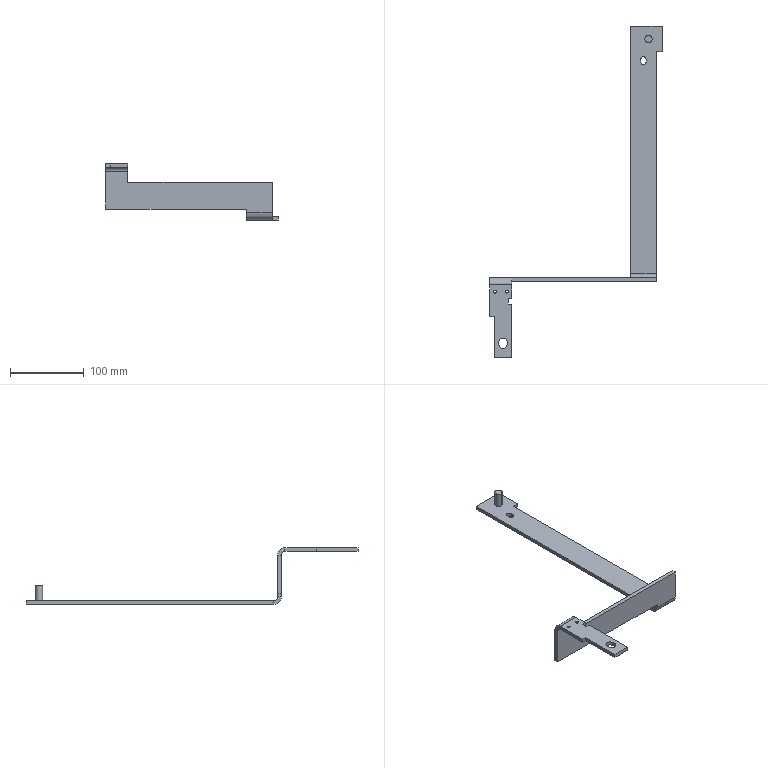Part | STEP file | 64562509 | 1 solid | 49 faces | box 233.8 x 450 x 76.5 mm | volume 121760 mm3 | plane 35 | cylinder 14 | commonest cylinder face diameters 4 x4 10 x4 7 x2 12 x2 20 x2